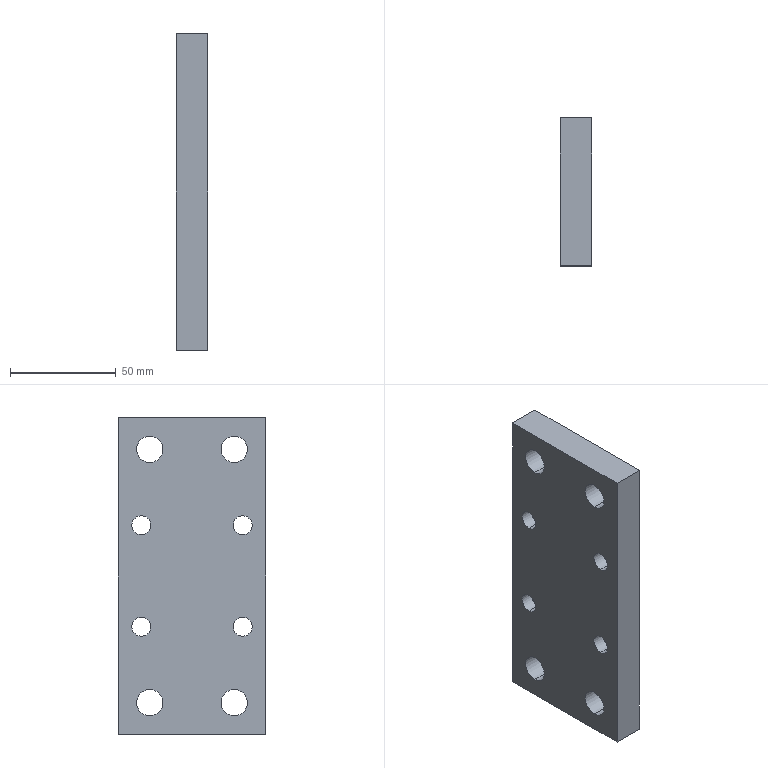Part | SolidWorks | features HoleWzd 2, Extrusion 1 | 1 solid | 34 faces | box 15 x 70 x 150 mm | volume 142248 mm3 | cylinder 24 | plane 10 | commonest cylinder face diameters 9 x8 12.5 x8 15 x8
STEP:
#1=CARTESIAN_POINT('',(15.,20.,-66.25));
#2=VERTEX_POINT('',#1);
#3=CARTESIAN_POINT('',(15.,20.,-53.75));
#4=VERTEX_POINT('',#3);
#5=CARTESIAN_POINT('',(15.,20.,-60.));
#6=DIRECTION('',(-1.,0.,0.));
#7=DIRECTION('',(0.,0.,1.));
#8=AXIS2_PLACEMENT_3D('',#5,#6,#7);
#9=CIRCLE('',#8,6.25);
#10=EDGE_CURVE('',#2,#4,#9,.T.);
#11=ORIENTED_EDGE('',*,*,#10,.F.);
#12=CARTESIAN_POINT('',(0.,20.,-66.25));
#13=VERTEX_POINT('',#12);
#14=CARTESIAN_POINT('',(0.,20.,-66.25));
#15=DIRECTION('',(-1.,0.,0.));
#16=VECTOR('',#15,1000.);
#17=LINE('',#14,#16);
#18=EDGE_CURVE('',#2,#13,#17,.T.);
#19=ORIENTED_EDGE('',*,*,#18,.T.);
#20=CARTESIAN_POINT('',(0.,20.,-53.75));
#21=VERTEX_POINT('',#20);
#22=CARTESIAN_POINT('',(0.,20.,-60.));
#23=DIRECTION('',(-1.,0.,0.));
#24=DIRECTION('',(0.,0.,1.));
#25=AXIS2_PLACEMENT_3D('',#22,#23,#24);
#26=CIRCLE('',#25,6.25);
#27=EDGE_CURVE('',#13,#21,#26,.T.);
#28=ORIENTED_EDGE('',*,*,#27,.T.);
#29=CARTESIAN_POINT('',(0.,20.,-53.75));
#30=DIRECTION('',(-1.,0.,0.));
#31=VECTOR('',#30,1000.);
#32=LINE('',#29,#31);
#33=EDGE_CURVE('',#4,#21,#32,.T.);
#34=ORIENTED_EDGE('',*,*,#33,.F.);
#35=EDGE_LOOP('',(#11,#19,#28,#34));
#36=FACE_OUTER_BOUND('',#35,.T.);
#37=CARTESIAN_POINT('',(0.,20.,-60.));
#38=DIRECTION('',(-1.,0.,0.));
#39=DIRECTION('',(0.,0.,1.));
#40=AXIS2_PLACEMENT_3D('',#37,#38,#39);
#41=CYLINDRICAL_SURFACE('',#40,6.25);
#42=ADVANCED_FACE('',(#36),#41,.F.);
#43=CARTESIAN_POINT('',(15.,-20.,-66.25));
#44=VERTEX_POINT('',#43);
#45=CARTESIAN_POINT('',(15.,-20.,-53.75));
#46=VERTEX_POINT('',#45);
#47=CARTESIAN_POINT('',(15.,-20.,-60.));
#48=DIRECTION('',(-1.,0.,0.));
#49=DIRECTION('',(0.,0.,1.));
#50=AXIS2_PLACEMENT_3D('',#47,#48,#49);
#51=CIRCLE('',#50,6.25);
#52=EDGE_CURVE('',#44,#46,#51,.T.);
#53=ORIENTED_EDGE('',*,*,#52,.F.);
#54=CARTESIAN_POINT('',(0.,-20.,-66.25));
#55=VERTEX_POINT('',#54);
#56=CARTESIAN_POINT('',(0.,-20.,-66.25));
#57=DIRECTION('',(-1.,0.,0.));
#58=VECTOR('',#57,1000.);
#59=LINE('',#56,#58);
#60=EDGE_CURVE('',#44,#55,#59,.T.);
#61=ORIENTED_EDGE('',*,*,#60,.T.);
#62=CARTESIAN_POINT('',(0.,-20.,-53.75));
#63=VERTEX_POINT('',#62);
#64=CARTESIAN_POINT('',(0.,-20.,-60.));
#65=DIRECTION('',(-1.,0.,0.));
#66=DIRECTION('',(0.,0.,1.));
#67=AXIS2_PLACEMENT_3D('',#64,#65,#66);
#68=CIRCLE('',#67,6.25);
#69=EDGE_CURVE('',#55,#63,#68,.T.);
#70=ORIENTED_EDGE('',*,*,#69,.T.);
#71=CARTESIAN_POINT('',(0.,-20.,-53.75));
#72=DIRECTION('',(-1.,0.,0.));
#73=VECTOR('',#72,1000.);
#74=LINE('',#71,#73);
#75=EDGE_CURVE('',#46,#63,#74,.T.);
#76=ORIENTED_EDGE('',*,*,#75,.F.);
#77=EDGE_LOOP('',(#53,#61,#70,#76));
#78=FACE_OUTER_BOUND('',#77,.T.);
#79=CARTESIAN_POINT('',(0.,-20.,-60.));
#80=DIRECTION('',(-1.,0.,0.));
#81=DIRECTION('',(0.,0.,1.));
#82=AXIS2_PLACEMENT_3D('',#79,#80,#81);
#83=CYLINDRICAL_SURFACE('',#82,6.25);
#84=ADVANCED_FACE('',(#78),#83,.F.);
#85=CARTESIAN_POINT('',(15.,20.,53.75));
#86=VERTEX_POINT('',#85);
#87=CARTESIAN_POINT('',(15.,20.,66.25));
#88=VERTEX_POINT('',#87);
#89=CARTESIAN_POINT('',(15.,20.,60.));
#90=DIRECTION('',(-1.,0.,0.));
#91=DIRECTION('',(0.,0.,1.));
#92=AXIS2_PLACEMENT_3D('',#89,#90,#91);
#93=CIRCLE('',#92,6.25);
#94=EDGE_CURVE('',#86,#88,#93,.T.);
#95=ORIENTED_EDGE('',*,*,#94,.F.);
#96=CARTESIAN_POINT('',(0.,20.,53.75));
#97=VERTEX_POINT('',#96);
#98=CARTESIAN_POINT('',(0.,20.,53.75));
#99=DIRECTION('',(-1.,0.,0.));
#100=VECTOR('',#99,1000.);
#101=LINE('',#98,#100);
#102=EDGE_CURVE('',#86,#97,#101,.T.);
#103=ORIENTED_EDGE('',*,*,#102,.T.);
#104=CARTESIAN_POINT('',(0.,20.,66.25));
#105=VERTEX_POINT('',#104);
#106=CARTESIAN_POINT('',(0.,20.,60.));
#107=DIRECTION('',(-1.,0.,0.));
#108=DIRECTION('',(0.,0.,1.));
#109=AXIS2_PLACEMENT_3D('',#106,#107,#108);
#110=CIRCLE('',#109,6.25);
#111=EDGE_CURVE('',#97,#105,#110,.T.);
#112=ORIENTED_EDGE('',*,*,#111,.T.);
#113=CARTESIAN_POINT('',(0.,20.,66.25));
#114=DIRECTION('',(-1.,0.,0.));
#115=VECTOR('',#114,1000.);
#116=LINE('',#113,#115);
#117=EDGE_CURVE('',#88,#105,#116,.T.);
#118=ORIENTED_EDGE('',*,*,#117,.F.);
#119=EDGE_LOOP('',(#95,#103,#112,#118));
#120=FACE_OUTER_BOUND('',#119,.T.);
#121=CARTESIAN_POINT('',(0.,20.,60.));
#122=DIRECTION('',(-1.,0.,0.));
#123=DIRECTION('',(0.,0.,1.));
#124=AXIS2_PLACEMENT_3D('',#121,#122,#123);
#125=CYLINDRICAL_SURFACE('',#124,6.25);
#126=ADVANCED_FACE('',(#120),#125,.F.);
#127=CARTESIAN_POINT('',(15.,-20.,53.75));
#128=VERTEX_POINT('',#127);
#129=CARTESIAN_POINT('',(15.,-20.,66.25));
#130=VERTEX_POINT('',#129);
#131=CARTESIAN_POINT('',(15.,-20.,60.));
#132=DIRECTION('',(-1.,0.,0.));
#133=DIRECTION('',(0.,0.,1.));
#134=AXIS2_PLACEMENT_3D('',#131,#132,#133);
#135=CIRCLE('',#134,6.25);
#136=EDGE_CURVE('',#128,#130,#135,.T.);
#137=ORIENTED_EDGE('',*,*,#136,.F.);
#138=CARTESIAN_POINT('',(0.,-20.,53.75));
#139=VERTEX_POINT('',#138);
#140=CARTESIAN_POINT('',(0.,-20.,53.75));
#141=DIRECTION('',(-1.,0.,0.));
#142=VECTOR('',#141,1000.);
#143=LINE('',#140,#142);
#144=EDGE_CURVE('',#128,#139,#143,.T.);
#145=ORIENTED_EDGE('',*,*,#144,.T.);
#146=CARTESIAN_POINT('',(0.,-20.,66.25));
#147=VERTEX_POINT('',#146);
#148=CARTESIAN_POINT('',(0.,-20.,60.));
#149=DIRECTION('',(-1.,0.,0.));
#150=DIRECTION('',(0.,0.,1.));
#151=AXIS2_PLACEMENT_3D('',#148,#149,#150);
#152=CIRCLE('',#151,6.25);
#153=EDGE_CURVE('',#139,#147,#152,.T.);
#154=ORIENTED_EDGE('',*,*,#153,.T.);
#155=CARTESIAN_POINT('',(0.,-20.,66.25));
#156=DIRECTION('',(-1.,0.,0.));
#157=VECTOR('',#156,1000.);
#158=LINE('',#155,#157);
#159=EDGE_CURVE('',#130,#147,#158,.T.);
#160=ORIENTED_EDGE('',*,*,#159,.F.);
#161=EDGE_LOOP('',(#137,#145,#154,#160));
#162=FACE_OUTER_BOUND('',#161,.T.);
#163=CARTESIAN_POINT('',(0.,-20.,60.));
#164=DIRECTION('',(-1.,0.,0.));
#165=DIRECTION('',(0.,0.,1.));
#166=AXIS2_PLACEMENT_3D('',#163,#164,#165);
#167=CYLINDRICAL_SURFACE('',#166,6.25);
#168=ADVANCED_FACE('',(#162),#167,.F.);
#169=CARTESIAN_POINT('',(6.,24.,31.5));
#170=VERTEX_POINT('',#169);
#171=CARTESIAN_POINT('',(6.,24.,16.5));
#172=VERTEX_POINT('',#171);
#173=CARTESIAN_POINT('',(6.,24.,24.));
#174=DIRECTION('',(1.,0.,0.));
#175=DIRECTION('',(0.,0.,-1.));
#176=AXIS2_PLACEMENT_3D('',#173,#174,#175);
#177=CIRCLE('',#176,7.5);
#178=EDGE_CURVE('',#170,#172,#177,.T.);
#179=ORIENTED_EDGE('',*,*,#178,.F.);
#180=CARTESIAN_POINT('',(15.,24.,31.5));
#181=VERTEX_POINT('',#180);
#182=CARTESIAN_POINT('',(15.,24.,31.5));
#183=DIRECTION('',(1.,0.,0.));
#184=VECTOR('',#183,1000.);
#185=LINE('',#182,#184);
#186=EDGE_CURVE('',#170,#181,#185,.T.);
#187=ORIENTED_EDGE('',*,*,#186,.T.);
#188=CARTESIAN_POINT('',(15.,24.,16.5));
#189=VERTEX_POINT('',#188);
#190=CARTESIAN_POINT('',(15.,24.,24.));
#191=DIRECTION('',(1.,0.,0.));
#192=DIRECTION('',(0.,0.,-1.));
#193=AXIS2_PLACEMENT_3D('',#190,#191,#192);
#194=CIRCLE('',#193,7.5);
#195=EDGE_CURVE('',#181,#189,#194,.T.);
#196=ORIENTED_EDGE('',*,*,#195,.T.);
#197=CARTESIAN_POINT('',(15.,24.,16.5));
#198=DIRECTION('',(1.,0.,0.));
#199=VECTOR('',#198,1000.);
#200=LINE('',#197,#199);
#201=EDGE_CURVE('',#172,#189,#200,.T.);
#202=ORIENTED_EDGE('',*,*,#201,.F.);
#203=EDGE_LOOP('',(#179,#187,#196,#202));
#204=FACE_OUTER_BOUND('',#203,.T.);
#205=CARTESIAN_POINT('',(15.,24.,24.));
#206=DIRECTION('',(1.,0.,0.));
#207=DIRECTION('',(0.,0.,-1.));
#208=AXIS2_PLACEMENT_3D('',#205,#206,#207);
#209=CYLINDRICAL_SURFACE('',#208,7.5);
#210=ADVANCED_FACE('',(#204),#209,.F.);
#211=CARTESIAN_POINT('',(0.,24.,28.5));
#212=VERTEX_POINT('',#211);
#213=CARTESIAN_POINT('',(0.,24.,19.5));
#214=VERTEX_POINT('',#213);
#215=CARTESIAN_POINT('',(0.,24.,24.));
#216=DIRECTION('',(1.,0.,0.));
#217=DIRECTION('',(0.,0.,-1.));
#218=AXIS2_PLACEMENT_3D('',#215,#216,#217);
#219=CIRCLE('',#218,4.5);
#220=EDGE_CURVE('',#212,#214,#219,.T.);
#221=ORIENTED_EDGE('',*,*,#220,.F.);
#222=CARTESIAN_POINT('',(6.,24.,28.5));
#223=VERTEX_POINT('',#222);
#224=CARTESIAN_POINT('',(15.,24.,28.5));
#225=DIRECTION('',(1.,0.,0.));
#226=VECTOR('',#225,1000.);
#227=LINE('',#224,#226);
#228=EDGE_CURVE('',#212,#223,#227,.T.);
#229=ORIENTED_EDGE('',*,*,#228,.T.);
#230=CARTESIAN_POINT('',(6.,24.,19.5));
#231=VERTEX_POINT('',#230);
#232=CARTESIAN_POINT('',(6.,24.,24.));
#233=DIRECTION('',(1.,0.,0.));
#234=DIRECTION('',(0.,0.,-1.));
#235=AXIS2_PLACEMENT_3D('',#232,#233,#234);
#236=CIRCLE('',#235,4.5);
#237=EDGE_CURVE('',#223,#231,#236,.T.);
#238=ORIENTED_EDGE('',*,*,#237,.T.);
#239=CARTESIAN_POINT('',(15.,24.,19.5));
#240=DIRECTION('',(1.,0.,0.));
#241=VECTOR('',#240,1000.);
#242=LINE('',#239,#241);
#243=EDGE_CURVE('',#214,#231,#242,.T.);
#244=ORIENTED_EDGE('',*,*,#243,.F.);
#245=EDGE_LOOP('',(#221,#229,#238,#244));
#246=FACE_OUTER_BOUND('',#245,.T.);
#247=CARTESIAN_POINT('',(15.,24.,24.));
#248=DIRECTION('',(1.,0.,0.));
#249=DIRECTION('',(0.,0.,-1.));
#250=AXIS2_PLACEMENT_3D('',#247,#248,#249);
#251=CYLINDRICAL_SURFACE('',#250,4.5);
#252=ADVANCED_FACE('',(#246),#251,.F.);
#253=CARTESIAN_POINT('',(6.,24.,-16.5));
#254=VERTEX_POINT('',#253);
#255=CARTESIAN_POINT('',(6.,24.,-31.5));
#256=VERTEX_POINT('',#255);
#257=CARTESIAN_POINT('',(6.,24.,-24.));
#258=DIRECTION('',(1.,0.,0.));
#259=DIRECTION('',(0.,0.,-1.));
#260=AXIS2_PLACEMENT_3D('',#257,#258,#259);
#261=CIRCLE('',#260,7.5);
#262=EDGE_CURVE('',#254,#256,#261,.T.);
#263=ORIENTED_EDGE('',*,*,#262,.F.);
#264=CARTESIAN_POINT('',(15.,24.,-16.5));
#265=VERTEX_POINT('',#264);
#266=CARTESIAN_POINT('',(15.,24.,-16.5));
#267=DIRECTION('',(1.,0.,0.));
#268=VECTOR('',#267,1000.);
#269=LINE('',#266,#268);
#270=EDGE_CURVE('',#254,#265,#269,.T.);
#271=ORIENTED_EDGE('',*,*,#270,.T.);
#272=CARTESIAN_POINT('',(15.,24.,-31.5));
#273=VERTEX_POINT('',#272);
#274=CARTESIAN_POINT('',(15.,24.,-24.));
#275=DIRECTION('',(1.,0.,0.));
#276=DIRECTION('',(0.,0.,-1.));
#277=AXIS2_PLACEMENT_3D('',#274,#275,#276);
#278=CIRCLE('',#277,7.5);
#279=EDGE_CURVE('',#265,#273,#278,.T.);
#280=ORIENTED_EDGE('',*,*,#279,.T.);
#281=CARTESIAN_POINT('',(15.,24.,-31.5));
#282=DIRECTION('',(1.,0.,0.));
#283=VECTOR('',#282,1000.);
#284=LINE('',#281,#283);
#285=EDGE_CURVE('',#256,#273,#284,.T.);
#286=ORIENTED_EDGE('',*,*,#285,.F.);
#287=EDGE_LOOP('',(#263,#271,#280,#286));
#288=FACE_OUTER_BOUND('',#287,.T.);
#289=CARTESIAN_POINT('',(15.,24.,-24.));
#290=DIRECTION('',(1.,0.,0.));
#291=DIRECTION('',(0.,0.,-1.));
#292=AXIS2_PLACEMENT_3D('',#289,#290,#291);
#293=CYLINDRICAL_SURFACE('',#292,7.5);
#294=ADVANCED_FACE('',(#288),#293,.F.);
#295=CARTESIAN_POINT('',(0.,24.,-19.5));
#296=VERTEX_POINT('',#295);
#297=CARTESIAN_POINT('',(0.,24.,-28.5));
#298=VERTEX_POINT('',#297);
#299=CARTESIAN_POINT('',(0.,24.,-24.));
#300=DIRECTION('',(1.,0.,0.));
#301=DIRECTION('',(0.,0.,-1.));
#302=AXIS2_PLACEMENT_3D('',#299,#300,#301);
#303=CIRCLE('',#302,4.5);
#304=EDGE_CURVE('',#296,#298,#303,.T.);
#305=ORIENTED_EDGE('',*,*,#304,.F.);
#306=CARTESIAN_POINT('',(6.,24.,-19.5));
#307=VERTEX_POINT('',#306);
#308=CARTESIAN_POINT('',(15.,24.,-19.5));
#309=DIRECTION('',(1.,0.,0.));
#310=VECTOR('',#309,1000.);
#311=LINE('',#308,#310);
#312=EDGE_CURVE('',#296,#307,#311,.T.);
#313=ORIENTED_EDGE('',*,*,#312,.T.);
#314=CARTESIAN_POINT('',(6.,24.,-28.5));
#315=VERTEX_POINT('',#314);
#316=CARTESIAN_POINT('',(6.,24.,-24.));
#317=DIRECTION('',(1.,0.,0.));
#318=DIRECTION('',(0.,0.,-1.));
#319=AXIS2_PLACEMENT_3D('',#316,#317,#318);
#320=CIRCLE('',#319,4.5);
#321=EDGE_CURVE('',#307,#315,#320,.T.);
#322=ORIENTED_EDGE('',*,*,#321,.T.);
#323=CARTESIAN_POINT('',(15.,24.,-28.5));
#324=DIRECTION('',(1.,0.,0.));
#325=VECTOR('',#324,1000.);
#326=LINE('',#323,#325);
#327=EDGE_CURVE('',#298,#315,#326,.T.);
#328=ORIENTED_EDGE('',*,*,#327,.F.);
#329=EDGE_LOOP('',(#305,#313,#322,#328));
#330=FACE_OUTER_BOUND('',#329,.T.);
#331=CARTESIAN_POINT('',(15.,24.,-24.));
#332=DIRECTION('',(1.,0.,0.));
#333=DIRECTION('',(0.,0.,-1.));
#334=AXIS2_PLACEMENT_3D('',#331,#332,#333);
#335=CYLINDRICAL_SURFACE('',#334,4.5);
#336=ADVANCED_FACE('',(#330),#335,.F.);
#337=CARTESIAN_POINT('',(6.,-24.,31.5));
#338=VERTEX_POINT('',#337);
#339=CARTESIAN_POINT('',(6.,-24.,16.5));
#340=VERTEX_POINT('',#339);
#341=CARTESIAN_POINT('',(6.,-24.,24.));
#342=DIRECTION('',(1.,0.,0.));
#343=DIRECTION('',(0.,0.,-1.));
#344=AXIS2_PLACEMENT_3D('',#341,#342,#343);
#345=CIRCLE('',#344,7.5);
#346=EDGE_CURVE('',#338,#340,#345,.T.);
#347=ORIENTED_EDGE('',*,*,#346,.F.);
#348=CARTESIAN_POINT('',(15.,-24.,31.5));
#349=VERTEX_POINT('',#348);
#350=CARTESIAN_POINT('',(15.,-24.,31.5));
#351=DIRECTION('',(1.,0.,0.));
#352=VECTOR('',#351,1000.);
#353=LINE('',#350,#352);
#354=EDGE_CURVE('',#338,#349,#353,.T.);
#355=ORIENTED_EDGE('',*,*,#354,.T.);
#356=CARTESIAN_POINT('',(15.,-24.,16.5));
#357=VERTEX_POINT('',#356);
#358=CARTESIAN_POINT('',(15.,-24.,24.));
#359=DIRECTION('',(1.,0.,0.));
#360=DIRECTION('',(0.,0.,-1.));
#361=AXIS2_PLACEMENT_3D('',#358,#359,#360);
#362=CIRCLE('',#361,7.5);
#363=EDGE_CURVE('',#349,#357,#362,.T.);
#364=ORIENTED_EDGE('',*,*,#363,.T.);
#365=CARTESIAN_POINT('',(15.,-24.,16.5));
#366=DIRECTION('',(1.,0.,0.));
#367=VECTOR('',#366,1000.);
#368=LINE('',#365,#367);
#369=EDGE_CURVE('',#340,#357,#368,.T.);
#370=ORIENTED_EDGE('',*,*,#369,.F.);
#371=EDGE_LOOP('',(#347,#355,#364,#370));
#372=FACE_OUTER_BOUND('',#371,.T.);
#373=CARTESIAN_POINT('',(15.,-24.,24.));
#374=DIRECTION('',(1.,0.,0.));
#375=DIRECTION('',(0.,0.,-1.));
#376=AXIS2_PLACEMENT_3D('',#373,#374,#375);
#377=CYLINDRICAL_SURFACE('',#376,7.5);
#378=ADVANCED_FACE('',(#372),#377,.F.);
#379=CARTESIAN_POINT('',(0.,-24.,28.5));
#380=VERTEX_POINT('',#379);
#381=CARTESIAN_POINT('',(0.,-24.,19.5));
#382=VERTEX_POINT('',#381);
#383=CARTESIAN_POINT('',(0.,-24.,24.));
#384=DIRECTION('',(1.,0.,0.));
#385=DIRECTION('',(0.,0.,-1.));
#386=AXIS2_PLACEMENT_3D('',#383,#384,#385);
#387=CIRCLE('',#386,4.5);
#388=EDGE_CURVE('',#380,#382,#387,.T.);
#389=ORIENTED_EDGE('',*,*,#388,.F.);
#390=CARTESIAN_POINT('',(6.,-24.,28.5));
#391=VERTEX_POINT('',#390);
#392=CARTESIAN_POINT('',(15.,-24.,28.5));
#393=DIRECTION('',(1.,0.,0.));
#394=VECTOR('',#393,1000.);
#395=LINE('',#392,#394);
#396=EDGE_CURVE('',#380,#391,#395,.T.);
#397=ORIENTED_EDGE('',*,*,#396,.T.);
#398=CARTESIAN_POINT('',(6.,-24.,19.5));
#399=VERTEX_POINT('',#398);
#400=CARTESIAN_POINT('',(6.,-24.,24.));
#401=DIRECTION('',(1.,0.,0.));
#402=DIRECTION('',(0.,0.,-1.));
#403=AXIS2_PLACEMENT_3D('',#400,#401,#402);
#404=CIRCLE('',#403,4.5);
#405=EDGE_CURVE('',#391,#399,#404,.T.);
#406=ORIENTED_EDGE('',*,*,#405,.T.);
#407=CARTESIAN_POINT('',(15.,-24.,19.5));
#408=DIRECTION('',(1.,0.,0.));
#409=VECTOR('',#408,1000.);
#410=LINE('',#407,#409);
#411=EDGE_CURVE('',#382,#399,#410,.T.);
#412=ORIENTED_EDGE('',*,*,#411,.F.);
#413=EDGE_LOOP('',(#389,#397,#406,#412));
#414=FACE_OUTER_BOUND('',#413,.T.);
#415=CARTESIAN_POINT('',(15.,-24.,24.));
#416=DIRECTION('',(1.,0.,0.));
#417=DIRECTION('',(0.,0.,-1.));
#418=AXIS2_PLACEMENT_3D('',#415,#416,#417);
#419=CYLINDRICAL_SURFACE('',#418,4.5);
#420=ADVANCED_FACE('',(#414),#419,.F.);
#421=CARTESIAN_POINT('',(6.,-24.,-16.5));
#422=VERTEX_POINT('',#421);
#423=CARTESIAN_POINT('',(6.,-24.,-31.5));
#424=VERTEX_POINT('',#423);
#425=CARTESIAN_POINT('',(6.,-24.,-24.));
#426=DIRECTION('',(1.,0.,0.));
#427=DIRECTION('',(0.,0.,-1.));
#428=AXIS2_PLACEMENT_3D('',#425,#426,#427);
#429=CIRCLE('',#428,7.5);
#430=EDGE_CURVE('',#422,#424,#429,.T.);
#431=ORIENTED_EDGE('',*,*,#430,.F.);
#432=CARTESIAN_POINT('',(15.,-24.,-16.5));
#433=VERTEX_POINT('',#432);
#434=CARTESIAN_POINT('',(15.,-24.,-16.5));
#435=DIRECTION('',(1.,0.,0.));
#436=VECTOR('',#435,1000.);
#437=LINE('',#434,#436);
#438=EDGE_CURVE('',#422,#433,#437,.T.);
#439=ORIENTED_EDGE('',*,*,#438,.T.);
#440=CARTESIAN_POINT('',(15.,-24.,-31.5));
#441=VERTEX_POINT('',#440);
#442=CARTESIAN_POINT('',(15.,-24.,-24.));
#443=DIRECTION('',(1.,0.,0.));
#444=DIRECTION('',(0.,0.,-1.));
#445=AXIS2_PLACEMENT_3D('',#442,#443,#444);
#446=CIRCLE('',#445,7.5);
#447=EDGE_CURVE('',#433,#441,#446,.T.);
#448=ORIENTED_EDGE('',*,*,#447,.T.);
#449=CARTESIAN_POINT('',(15.,-24.,-31.5));
#450=DIRECTION('',(1.,0.,0.));
#451=VECTOR('',#450,1000.);
#452=LINE('',#449,#451);
#453=EDGE_CURVE('',#424,#441,#452,.T.);
#454=ORIENTED_EDGE('',*,*,#453,.F.);
#455=EDGE_LOOP('',(#431,#439,#448,#454));
#456=FACE_OUTER_BOUND('',#455,.T.);
#457=CARTESIAN_POINT('',(15.,-24.,-24.));
#458=DIRECTION('',(1.,0.,0.));
#459=DIRECTION('',(0.,0.,-1.));
#460=AXIS2_PLACEMENT_3D('',#457,#458,#459);
#461=CYLINDRICAL_SURFACE('',#460,7.5);
#462=ADVANCED_FACE('',(#456),#461,.F.);
#463=CARTESIAN_POINT('',(0.,-24.,-19.5));
#464=VERTEX_POINT('',#463);
#465=CARTESIAN_POINT('',(0.,-24.,-28.5));
#466=VERTEX_POINT('',#465);
#467=CARTESIAN_POINT('',(0.,-24.,-24.));
#468=DIRECTION('',(1.,0.,0.));
#469=DIRECTION('',(0.,0.,-1.));
#470=AXIS2_PLACEMENT_3D('',#467,#468,#469);
#471=CIRCLE('',#470,4.5);
#472=EDGE_CURVE('',#464,#466,#471,.T.);
#473=ORIENTED_EDGE('',*,*,#472,.F.);
#474=CARTESIAN_POINT('',(6.,-24.,-19.5));
#475=VERTEX_POINT('',#474);
#476=CARTESIAN_POINT('',(15.,-24.,-19.5));
#477=DIRECTION('',(1.,0.,0.));
#478=VECTOR('',#477,1000.);
#479=LINE('',#476,#478);
#480=EDGE_CURVE('',#464,#475,#479,.T.);
#481=ORIENTED_EDGE('',*,*,#480,.T.);
#482=CARTESIAN_POINT('',(6.,-24.,-28.5));
#483=VERTEX_POINT('',#482);
#484=CARTESIAN_POINT('',(6.,-24.,-24.));
#485=DIRECTION('',(1.,0.,0.));
#486=DIRECTION('',(0.,0.,-1.));
#487=AXIS2_PLACEMENT_3D('',#484,#485,#486);
#488=CIRCLE('',#487,4.5);
#489=EDGE_CURVE('',#475,#483,#488,.T.);
#490=ORIENTED_EDGE('',*,*,#489,.T.);
#491=CARTESIAN_POINT('',(15.,-24.,-28.5));
#492=DIRECTION('',(1.,0.,0.));
#493=VECTOR('',#492,1000.);
#494=LINE('',#491,#493);
#495=EDGE_CURVE('',#466,#483,#494,.T.);
#496=ORIENTED_EDGE('',*,*,#495,.F.);
#497=EDGE_LOOP('',(#473,#481,#490,#496));
#498=FACE_OUTER_BOUND('',#497,.T.);
#499=CARTESIAN_POINT('',(15.,-24.,-24.));
#500=DIRECTION('',(1.,0.,0.));
#501=DIRECTION('',(0.,0.,-1.));
#502=AXIS2_PLACEMENT_3D('',#499,#500,#501);
#503=CYLINDRICAL_SURFACE('',#502,4.5);
#504=ADVANCED_FACE('',(#498),#503,.F.);
#505=CARTESIAN_POINT('',(0.,-35.,-75.));
#506=VERTEX_POINT('',#505);
#507=CARTESIAN_POINT('',(0.,35.,-75.));
#508=VERTEX_POINT('',#507);
#509=CARTESIAN_POINT('',(0.,35.,-75.));
#510=DIRECTION('',(0.,1.,0.));
#511=VECTOR('',#510,1000.);
#512=LINE('',#509,#511);
#513=EDGE_CURVE('',#506,#508,#512,.T.);
#514=ORIENTED_EDGE('',*,*,#513,.T.);
#515=CARTESIAN_POINT('',(15.,35.,-75.));
#516=VERTEX_POINT('',#515);
#517=CARTESIAN_POINT('',(15.,35.,-75.));
#518=DIRECTION('',(-1.,0.,0.));
#519=VECTOR('',#518,1000.);
#520=LINE('',#517,#519);
#521=EDGE_CURVE('',#516,#508,#520,.T.);
#522=ORIENTED_EDGE('',*,*,#521,.F.);
#523=CARTESIAN_POINT('',(15.,-35.,-75.));
#524=VERTEX_POINT('',#523);
#525=CARTESIAN_POINT('',(15.,35.,-75.));
#526=DIRECTION('',(0.,1.,0.));
#527=VECTOR('',#526,1000.);
#528=LINE('',#525,#527);
#529=EDGE_CURVE('',#524,#516,#528,.T.);
#530=ORIENTED_EDGE('',*,*,#529,.F.);
#531=CARTESIAN_POINT('',(15.,-35.,-75.));
#532=DIRECTION('',(-1.,0.,0.));
#533=VECTOR('',#532,1000.);
#534=LINE('',#531,#533);
#535=EDGE_CURVE('',#524,#506,#534,.T.);
#536=ORIENTED_EDGE('',*,*,#535,.T.);
#537=EDGE_LOOP('',(#514,#522,#530,#536));
#538=FACE_OUTER_BOUND('',#537,.T.);
#539=CARTESIAN_POINT('',(15.,35.,-75.));
#540=DIRECTION('',(0.,0.,1.));
#541=DIRECTION('',(0.,-1.,0.));
#542=AXIS2_PLACEMENT_3D('',#539,#540,#541);
#543=PLANE('',#542);
#544=ADVANCED_FACE('',(#538),#543,.F.);
#545=CARTESIAN_POINT('',(0.,35.,75.));
#546=VERTEX_POINT('',#545);
#547=CARTESIAN_POINT('',(0.,35.,75.));
#548=DIRECTION('',(0.,0.,1.));
#549=VECTOR('',#548,1000.);
#550=LINE('',#547,#549);
#551=EDGE_CURVE('',#508,#546,#550,.T.);
#552=ORIENTED_EDGE('',*,*,#551,.T.);
#553=CARTESIAN_POINT('',(15.,35.,75.));
#554=VERTEX_POINT('',#553);
#555=CARTESIAN_POINT('',(15.,35.,75.));
#556=DIRECTION('',(-1.,0.,0.));
#557=VECTOR('',#556,1000.);
#558=LINE('',#555,#557);
#559=EDGE_CURVE('',#554,#546,#558,.T.);
#560=ORIENTED_EDGE('',*,*,#559,.F.);
#561=CARTESIAN_POINT('',(15.,35.,75.));
#562=DIRECTION('',(0.,0.,1.));
#563=VECTOR('',#562,1000.);
#564=LINE('',#561,#563);
#565=EDGE_CURVE('',#516,#554,#564,.T.);
#566=ORIENTED_EDGE('',*,*,#565,.F.);
#567=ORIENTED_EDGE('',*,*,#521,.T.);
#568=EDGE_LOOP('',(#552,#560,#566,#567));
#569=FACE_OUTER_BOUND('',#568,.T.);
#570=CARTESIAN_POINT('',(15.,35.,75.));
#571=DIRECTION('',(0.,-1.,0.));
#572=DIRECTION('',(0.,0.,-1.));
#573=AXIS2_PLACEMENT_3D('',#570,#571,#572);
#574=PLANE('',#573);
#575=ADVANCED_FACE('',(#569),#574,.F.);
#576=CARTESIAN_POINT('',(0.,-35.,75.));
#577=VERTEX_POINT('',#576);
#578=CARTESIAN_POINT('',(0.,35.,75.));
#579=DIRECTION('',(0.,-1.,0.));
#580=VECTOR('',#579,1000.);
#581=LINE('',#578,#580);
#582=EDGE_CURVE('',#546,#577,#581,.T.);
#583=ORIENTED_EDGE('',*,*,#582,.T.);
#584=CARTESIAN_POINT('',(15.,-35.,75.));
#585=VERTEX_POINT('',#584);
#586=CARTESIAN_POINT('',(15.,-35.,75.));
#587=DIRECTION('',(-1.,0.,0.));
#588=VECTOR('',#587,1000.);
#589=LINE('',#586,#588);
#590=EDGE_CURVE('',#585,#577,#589,.T.);
#591=ORIENTED_EDGE('',*,*,#590,.F.);
#592=CARTESIAN_POINT('',(15.,35.,75.));
#593=DIRECTION('',(0.,-1.,0.));
#594=VECTOR('',#593,1000.);
#595=LINE('',#592,#594);
#596=EDGE_CURVE('',#554,#585,#595,.T.);
#597=ORIENTED_EDGE('',*,*,#596,.F.);
#598=ORIENTED_EDGE('',*,*,#559,.T.);
#599=EDGE_LOOP('',(#583,#591,#597,#598));
#600=FACE_OUTER_BOUND('',#599,.T.);
#601=CARTESIAN_POINT('',(15.,35.,75.));
#602=DIRECTION('',(0.,0.,-1.));
#603=DIRECTION('',(0.,1.,0.));
#604=AXIS2_PLACEMENT_3D('',#601,#602,#603);
#605=PLANE('',#604);
#606=ADVANCED_FACE('',(#600),#605,.F.);
#607=CARTESIAN_POINT('',(0.,-35.,75.));
#608=DIRECTION('',(0.,0.,-1.));
#609=VECTOR('',#608,1000.);
#610=LINE('',#607,#609);
#611=EDGE_CURVE('',#577,#506,#610,.T.);
#612=ORIENTED_EDGE('',*,*,#611,.T.);
#613=ORIENTED_EDGE('',*,*,#535,.F.);
#614=CARTESIAN_POINT('',(15.,-35.,75.));
#615=DIRECTION('',(0.,0.,-1.));
#616=VECTOR('',#615,1000.);
#617=LINE('',#614,#616);
#618=EDGE_CURVE('',#585,#524,#617,.T.);
#619=ORIENTED_EDGE('',*,*,#618,.F.);
#620=ORIENTED_EDGE('',*,*,#590,.T.);
#621=EDGE_LOOP('',(#612,#613,#619,#620));
#622=FACE_OUTER_BOUND('',#621,.T.);
#623=CARTESIAN_POINT('',(15.,-35.,75.));
#624=DIRECTION('',(0.,1.,0.));
#625=DIRECTION('',(0.,0.,1.));
#626=AXIS2_PLACEMENT_3D('',#623,#624,#625);
#627=PLANE('',#626);
#628=ADVANCED_FACE('',(#622),#627,.F.);
#629=CARTESIAN_POINT('',(15.,20.,-60.));
#630=DIRECTION('',(-1.,0.,0.));
#631=DIRECTION('',(0.,0.,1.));
#632=AXIS2_PLACEMENT_3D('',#629,#630,#631);
#633=CIRCLE('',#632,6.25);
#634=EDGE_CURVE('',#4,#2,#633,.T.);
#635=ORIENTED_EDGE('',*,*,#634,.T.);
#636=ORIENTED_EDGE('',*,*,#10,.T.);
#637=EDGE_LOOP('',(#635,#636));
#638=FACE_BOUND('',#637,.T.);
#639=CARTESIAN_POINT('',(15.,-20.,-60.));
#640=DIRECTION('',(-1.,0.,0.));
#641=DIRECTION('',(0.,0.,1.));
#642=AXIS2_PLACEMENT_3D('',#639,#640,#641);
#643=CIRCLE('',#642,6.25);
#644=EDGE_CURVE('',#46,#44,#643,.T.);
#645=ORIENTED_EDGE('',*,*,#644,.T.);
#646=ORIENTED_EDGE('',*,*,#52,.T.);
#647=EDGE_LOOP('',(#645,#646));
#648=FACE_BOUND('',#647,.T.);
#649=CARTESIAN_POINT('',(15.,20.,60.));
#650=DIRECTION('',(-1.,0.,0.));
#651=DIRECTION('',(0.,0.,1.));
#652=AXIS2_PLACEMENT_3D('',#649,#650,#651);
#653=CIRCLE('',#652,6.25);
#654=EDGE_CURVE('',#88,#86,#653,.T.);
#655=ORIENTED_EDGE('',*,*,#654,.T.);
#656=ORIENTED_EDGE('',*,*,#94,.T.);
#657=EDGE_LOOP('',(#655,#656));
#658=FACE_BOUND('',#657,.T.);
#659=CARTESIAN_POINT('',(15.,-20.,60.));
#660=DIRECTION('',(-1.,0.,0.));
#661=DIRECTION('',(0.,0.,1.));
#662=AXIS2_PLACEMENT_3D('',#659,#660,#661);
#663=CIRCLE('',#662,6.25);
#664=EDGE_CURVE('',#130,#128,#663,.T.);
#665=ORIENTED_EDGE('',*,*,#664,.T.);
#666=ORIENTED_EDGE('',*,*,#136,.T.);
#667=EDGE_LOOP('',(#665,#666));
#668=FACE_BOUND('',#667,.T.);
#669=CARTESIAN_POINT('',(15.,24.,24.));
#670=DIRECTION('',(1.,0.,0.));
#671=DIRECTION('',(0.,0.,-1.));
#672=AXIS2_PLACEMENT_3D('',#669,#670,#671);
#673=CIRCLE('',#672,7.5);
#674=EDGE_CURVE('',#189,#181,#673,.T.);
#675=ORIENTED_EDGE('',*,*,#674,.F.);
#676=ORIENTED_EDGE('',*,*,#195,.F.);
#677=EDGE_LOOP('',(#675,#676));
#678=FACE_BOUND('',#677,.T.);
#679=CARTESIAN_POINT('',(15.,24.,-24.));
#680=DIRECTION('',(1.,0.,0.));
#681=DIRECTION('',(0.,0.,-1.));
#682=AXIS2_PLACEMENT_3D('',#679,#680,#681);
#683=CIRCLE('',#682,7.5);
#684=EDGE_CURVE('',#273,#265,#683,.T.);
#685=ORIENTED_EDGE('',*,*,#684,.F.);
#686=ORIENTED_EDGE('',*,*,#279,.F.);
#687=EDGE_LOOP('',(#685,#686));
#688=FACE_BOUND('',#687,.T.);
#689=CARTESIAN_POINT('',(15.,-24.,24.));
#690=DIRECTION('',(1.,0.,0.));
#691=DIRECTION('',(0.,0.,-1.));
#692=AXIS2_PLACEMENT_3D('',#689,#690,#691);
#693=CIRCLE('',#692,7.5);
#694=EDGE_CURVE('',#357,#349,#693,.T.);
#695=ORIENTED_EDGE('',*,*,#694,.F.);
#696=ORIENTED_EDGE('',*,*,#363,.F.);
#697=EDGE_LOOP('',(#695,#696));
#698=FACE_BOUND('',#697,.T.);
#699=CARTESIAN_POINT('',(15.,-24.,-24.));
#700=DIRECTION('',(1.,0.,0.));
#701=DIRECTION('',(0.,0.,-1.));
#702=AXIS2_PLACEMENT_3D('',#699,#700,#701);
#703=CIRCLE('',#702,7.5);
#704=EDGE_CURVE('',#441,#433,#703,.T.);
#705=ORIENTED_EDGE('',*,*,#704,.F.);
#706=ORIENTED_EDGE('',*,*,#447,.F.);
#707=EDGE_LOOP('',(#705,#706));
#708=FACE_BOUND('',#707,.T.);
#709=ORIENTED_EDGE('',*,*,#529,.T.);
#710=ORIENTED_EDGE('',*,*,#565,.T.);
#711=ORIENTED_EDGE('',*,*,#596,.T.);
#712=ORIENTED_EDGE('',*,*,#618,.T.);
#713=EDGE_LOOP('',(#709,#710,#711,#712));
#714=FACE_OUTER_BOUND('',#713,.T.);
#715=CARTESIAN_POINT('',(15.,0.,0.));
#716=DIRECTION('',(1.,0.,0.));
#717=DIRECTION('',(0.,0.,-1.));
#718=AXIS2_PLACEMENT_3D('',#715,#716,#717);
#719=PLANE('',#718);
#720=ADVANCED_FACE('',(#638,#648,#658,#668,#678,#688,#698,#708,#714),#719,.T.);
#721=CARTESIAN_POINT('',(0.,20.,-60.));
#722=DIRECTION('',(-1.,0.,0.));
#723=DIRECTION('',(0.,0.,1.));
#724=AXIS2_PLACEMENT_3D('',#721,#722,#723);
#725=CIRCLE('',#724,6.25);
#726=EDGE_CURVE('',#21,#13,#725,.T.);
#727=ORIENTED_EDGE('',*,*,#726,.F.);
#728=ORIENTED_EDGE('',*,*,#27,.F.);
#729=EDGE_LOOP('',(#727,#728));
#730=FACE_BOUND('',#729,.T.);
#731=CARTESIAN_POINT('',(0.,-20.,-60.));
#732=DIRECTION('',(-1.,0.,0.));
#733=DIRECTION('',(0.,0.,1.));
#734=AXIS2_PLACEMENT_3D('',#731,#732,#733);
#735=CIRCLE('',#734,6.25);
#736=EDGE_CURVE('',#63,#55,#735,.T.);
#737=ORIENTED_EDGE('',*,*,#736,.F.);
#738=ORIENTED_EDGE('',*,*,#69,.F.);
#739=EDGE_LOOP('',(#737,#738));
#740=FACE_BOUND('',#739,.T.);
#741=CARTESIAN_POINT('',(0.,20.,60.));
#742=DIRECTION('',(-1.,0.,0.));
#743=DIRECTION('',(0.,0.,1.));
#744=AXIS2_PLACEMENT_3D('',#741,#742,#743);
#745=CIRCLE('',#744,6.25);
#746=EDGE_CURVE('',#105,#97,#745,.T.);
#747=ORIENTED_EDGE('',*,*,#746,.F.);
#748=ORIENTED_EDGE('',*,*,#111,.F.);
#749=EDGE_LOOP('',(#747,#748));
#750=FACE_BOUND('',#749,.T.);
#751=CARTESIAN_POINT('',(0.,-20.,60.));
#752=DIRECTION('',(-1.,0.,0.));
#753=DIRECTION('',(0.,0.,1.));
#754=AXIS2_PLACEMENT_3D('',#751,#752,#753);
#755=CIRCLE('',#754,6.25);
#756=EDGE_CURVE('',#147,#139,#755,.T.);
#757=ORIENTED_EDGE('',*,*,#756,.F.);
#758=ORIENTED_EDGE('',*,*,#153,.F.);
#759=EDGE_LOOP('',(#757,#758));
#760=FACE_BOUND('',#759,.T.);
#761=CARTESIAN_POINT('',(0.,24.,24.));
#762=DIRECTION('',(1.,0.,0.));
#763=DIRECTION('',(0.,0.,-1.));
#764=AXIS2_PLACEMENT_3D('',#761,#762,#763);
#765=CIRCLE('',#764,4.5);
#766=EDGE_CURVE('',#214,#212,#765,.T.);
#767=ORIENTED_EDGE('',*,*,#766,.T.);
#768=ORIENTED_EDGE('',*,*,#220,.T.);
#769=EDGE_LOOP('',(#767,#768));
#770=FACE_BOUND('',#769,.T.);
#771=CARTESIAN_POINT('',(0.,24.,-24.));
#772=DIRECTION('',(1.,0.,0.));
#773=DIRECTION('',(0.,0.,-1.));
#774=AXIS2_PLACEMENT_3D('',#771,#772,#773);
#775=CIRCLE('',#774,4.5);
#776=EDGE_CURVE('',#298,#296,#775,.T.);
#777=ORIENTED_EDGE('',*,*,#776,.T.);
#778=ORIENTED_EDGE('',*,*,#304,.T.);
#779=EDGE_LOOP('',(#777,#778));
#780=FACE_BOUND('',#779,.T.);
#781=CARTESIAN_POINT('',(0.,-24.,24.));
#782=DIRECTION('',(1.,0.,0.));
#783=DIRECTION('',(0.,0.,-1.));
#784=AXIS2_PLACEMENT_3D('',#781,#782,#783);
#785=CIRCLE('',#784,4.5);
#786=EDGE_CURVE('',#382,#380,#785,.T.);
#787=ORIENTED_EDGE('',*,*,#786,.T.);
#788=ORIENTED_EDGE('',*,*,#388,.T.);
#789=EDGE_LOOP('',(#787,#788));
#790=FACE_BOUND('',#789,.T.);
#791=CARTESIAN_POINT('',(0.,-24.,-24.));
#792=DIRECTION('',(1.,0.,0.));
#793=DIRECTION('',(0.,0.,-1.));
#794=AXIS2_PLACEMENT_3D('',#791,#792,#793);
#795=CIRCLE('',#794,4.5);
#796=EDGE_CURVE('',#466,#464,#795,.T.);
#797=ORIENTED_EDGE('',*,*,#796,.T.);
#798=ORIENTED_EDGE('',*,*,#472,.T.);
#799=EDGE_LOOP('',(#797,#798));
#800=FACE_BOUND('',#799,.T.);
#801=ORIENTED_EDGE('',*,*,#513,.F.);
#802=ORIENTED_EDGE('',*,*,#611,.F.);
#803=ORIENTED_EDGE('',*,*,#582,.F.);
#804=ORIENTED_EDGE('',*,*,#551,.F.);
#805=EDGE_LOOP('',(#801,#802,#803,#804));
#806=FACE_OUTER_BOUND('',#805,.T.);
#807=CARTESIAN_POINT('',(0.,0.,0.));
#808=DIRECTION('',(1.,0.,0.));
#809=DIRECTION('',(0.,0.,-1.));
#810=AXIS2_PLACEMENT_3D('',#807,#808,#809);
#811=PLANE('',#810);
#812=ADVANCED_FACE('',(#730,#740,#750,#760,#770,#780,#790,#800,#806),#811,.F.);
#813=ORIENTED_EDGE('',*,*,#480,.F.);
#814=ORIENTED_EDGE('',*,*,#796,.F.);
#815=ORIENTED_EDGE('',*,*,#495,.T.);
#816=CARTESIAN_POINT('',(6.,-24.,-24.));
#817=DIRECTION('',(1.,0.,0.));
#818=DIRECTION('',(0.,0.,-1.));
#819=AXIS2_PLACEMENT_3D('',#816,#817,#818);
#820=CIRCLE('',#819,4.5);
#821=EDGE_CURVE('',#483,#475,#820,.T.);
#822=ORIENTED_EDGE('',*,*,#821,.T.);
#823=EDGE_LOOP('',(#813,#814,#815,#822));
#824=FACE_OUTER_BOUND('',#823,.T.);
#825=CARTESIAN_POINT('',(15.,-24.,-24.));
#826=DIRECTION('',(1.,0.,0.));
#827=DIRECTION('',(0.,0.,-1.));
#828=AXIS2_PLACEMENT_3D('',#825,#826,#827);
#829=CYLINDRICAL_SURFACE('',#828,4.5);
#830=ADVANCED_FACE('',(#824),#829,.F.);
#831=ORIENTED_EDGE('',*,*,#821,.F.);
#832=ORIENTED_EDGE('',*,*,#489,.F.);
#833=EDGE_LOOP('',(#831,#832));
#834=FACE_BOUND('',#833,.T.);
#835=CARTESIAN_POINT('',(6.,-24.,-24.));
#836=DIRECTION('',(1.,0.,0.));
#837=DIRECTION('',(0.,0.,-1.));
#838=AXIS2_PLACEMENT_3D('',#835,#836,#837);
#839=CIRCLE('',#838,7.5);
#840=EDGE_CURVE('',#424,#422,#839,.T.);
#841=ORIENTED_EDGE('',*,*,#840,.T.);
#842=ORIENTED_EDGE('',*,*,#430,.T.);
#843=EDGE_LOOP('',(#841,#842));
#844=FACE_OUTER_BOUND('',#843,.T.);
#845=CARTESIAN_POINT('',(6.,-19.5,-24.));
#846=DIRECTION('',(-1.,0.,0.));
#847=DIRECTION('',(0.,0.,1.));
#848=AXIS2_PLACEMENT_3D('',#845,#846,#847);
#849=PLANE('',#848);
#850=ADVANCED_FACE('',(#834,#844),#849,.F.);
#851=ORIENTED_EDGE('',*,*,#438,.F.);
#852=ORIENTED_EDGE('',*,*,#840,.F.);
#853=ORIENTED_EDGE('',*,*,#453,.T.);
#854=ORIENTED_EDGE('',*,*,#704,.T.);
#855=EDGE_LOOP('',(#851,#852,#853,#854));
#856=FACE_OUTER_BOUND('',#855,.T.);
#857=CARTESIAN_POINT('',(15.,-24.,-24.));
#858=DIRECTION('',(1.,0.,0.));
#859=DIRECTION('',(0.,0.,-1.));
#860=AXIS2_PLACEMENT_3D('',#857,#858,#859);
#861=CYLINDRICAL_SURFACE('',#860,7.5);
#862=ADVANCED_FACE('',(#856),#861,.F.);
#863=ORIENTED_EDGE('',*,*,#396,.F.);
#864=ORIENTED_EDGE('',*,*,#786,.F.);
#865=ORIENTED_EDGE('',*,*,#411,.T.);
#866=CARTESIAN_POINT('',(6.,-24.,24.));
#867=DIRECTION('',(1.,0.,0.));
#868=DIRECTION('',(0.,0.,-1.));
#869=AXIS2_PLACEMENT_3D('',#866,#867,#868);
#870=CIRCLE('',#869,4.5);
#871=EDGE_CURVE('',#399,#391,#870,.T.);
#872=ORIENTED_EDGE('',*,*,#871,.T.);
#873=EDGE_LOOP('',(#863,#864,#865,#872));
#874=FACE_OUTER_BOUND('',#873,.T.);
#875=CARTESIAN_POINT('',(15.,-24.,24.));
#876=DIRECTION('',(1.,0.,0.));
#877=DIRECTION('',(0.,0.,-1.));
#878=AXIS2_PLACEMENT_3D('',#875,#876,#877);
#879=CYLINDRICAL_SURFACE('',#878,4.5);
#880=ADVANCED_FACE('',(#874),#879,.F.);
#881=ORIENTED_EDGE('',*,*,#871,.F.);
#882=ORIENTED_EDGE('',*,*,#405,.F.);
#883=EDGE_LOOP('',(#881,#882));
#884=FACE_BOUND('',#883,.T.);
#885=CARTESIAN_POINT('',(6.,-24.,24.));
#886=DIRECTION('',(1.,0.,0.));
#887=DIRECTION('',(0.,0.,-1.));
#888=AXIS2_PLACEMENT_3D('',#885,#886,#887);
#889=CIRCLE('',#888,7.5);
#890=EDGE_CURVE('',#340,#338,#889,.T.);
#891=ORIENTED_EDGE('',*,*,#890,.T.);
#892=ORIENTED_EDGE('',*,*,#346,.T.);
#893=EDGE_LOOP('',(#891,#892));
#894=FACE_OUTER_BOUND('',#893,.T.);
#895=CARTESIAN_POINT('',(6.,-19.5,24.));
#896=DIRECTION('',(-1.,0.,0.));
#897=DIRECTION('',(0.,0.,1.));
#898=AXIS2_PLACEMENT_3D('',#895,#896,#897);
#899=PLANE('',#898);
#900=ADVANCED_FACE('',(#884,#894),#899,.F.);
#901=ORIENTED_EDGE('',*,*,#354,.F.);
#902=ORIENTED_EDGE('',*,*,#890,.F.);
#903=ORIENTED_EDGE('',*,*,#369,.T.);
#904=ORIENTED_EDGE('',*,*,#694,.T.);
#905=EDGE_LOOP('',(#901,#902,#903,#904));
#906=FACE_OUTER_BOUND('',#905,.T.);
#907=CARTESIAN_POINT('',(15.,-24.,24.));
#908=DIRECTION('',(1.,0.,0.));
#909=DIRECTION('',(0.,0.,-1.));
#910=AXIS2_PLACEMENT_3D('',#907,#908,#909);
#911=CYLINDRICAL_SURFACE('',#910,7.5);
#912=ADVANCED_FACE('',(#906),#911,.F.);
#913=ORIENTED_EDGE('',*,*,#312,.F.);
#914=ORIENTED_EDGE('',*,*,#776,.F.);
#915=ORIENTED_EDGE('',*,*,#327,.T.);
#916=CARTESIAN_POINT('',(6.,24.,-24.));
#917=DIRECTION('',(1.,0.,0.));
#918=DIRECTION('',(0.,0.,-1.));
#919=AXIS2_PLACEMENT_3D('',#916,#917,#918);
#920=CIRCLE('',#919,4.5);
#921=EDGE_CURVE('',#315,#307,#920,.T.);
#922=ORIENTED_EDGE('',*,*,#921,.T.);
#923=EDGE_LOOP('',(#913,#914,#915,#922));
#924=FACE_OUTER_BOUND('',#923,.T.);
#925=CARTESIAN_POINT('',(15.,24.,-24.));
#926=DIRECTION('',(1.,0.,0.));
#927=DIRECTION('',(0.,0.,-1.));
#928=AXIS2_PLACEMENT_3D('',#925,#926,#927);
#929=CYLINDRICAL_SURFACE('',#928,4.5);
#930=ADVANCED_FACE('',(#924),#929,.F.);
#931=ORIENTED_EDGE('',*,*,#921,.F.);
#932=ORIENTED_EDGE('',*,*,#321,.F.);
#933=EDGE_LOOP('',(#931,#932));
#934=FACE_BOUND('',#933,.T.);
#935=CARTESIAN_POINT('',(6.,24.,-24.));
#936=DIRECTION('',(1.,0.,0.));
#937=DIRECTION('',(0.,0.,-1.));
#938=AXIS2_PLACEMENT_3D('',#935,#936,#937);
#939=CIRCLE('',#938,7.5);
#940=EDGE_CURVE('',#256,#254,#939,.T.);
#941=ORIENTED_EDGE('',*,*,#940,.T.);
#942=ORIENTED_EDGE('',*,*,#262,.T.);
#943=EDGE_LOOP('',(#941,#942));
#944=FACE_OUTER_BOUND('',#943,.T.);
#945=CARTESIAN_POINT('',(6.,28.5,-24.));
#946=DIRECTION('',(-1.,0.,0.));
#947=DIRECTION('',(0.,0.,1.));
#948=AXIS2_PLACEMENT_3D('',#945,#946,#947);
#949=PLANE('',#948);
#950=ADVANCED_FACE('',(#934,#944),#949,.F.);
#951=ORIENTED_EDGE('',*,*,#270,.F.);
#952=ORIENTED_EDGE('',*,*,#940,.F.);
#953=ORIENTED_EDGE('',*,*,#285,.T.);
#954=ORIENTED_EDGE('',*,*,#684,.T.);
#955=EDGE_LOOP('',(#951,#952,#953,#954));
#956=FACE_OUTER_BOUND('',#955,.T.);
#957=CARTESIAN_POINT('',(15.,24.,-24.));
#958=DIRECTION('',(1.,0.,0.));
#959=DIRECTION('',(0.,0.,-1.));
#960=AXIS2_PLACEMENT_3D('',#957,#958,#959);
#961=CYLINDRICAL_SURFACE('',#960,7.5);
#962=ADVANCED_FACE('',(#956),#961,.F.);
#963=ORIENTED_EDGE('',*,*,#228,.F.);
#964=ORIENTED_EDGE('',*,*,#766,.F.);
#965=ORIENTED_EDGE('',*,*,#243,.T.);
#966=CARTESIAN_POINT('',(6.,24.,24.));
#967=DIRECTION('',(1.,0.,0.));
#968=DIRECTION('',(0.,0.,-1.));
#969=AXIS2_PLACEMENT_3D('',#966,#967,#968);
#970=CIRCLE('',#969,4.5);
#971=EDGE_CURVE('',#231,#223,#970,.T.);
#972=ORIENTED_EDGE('',*,*,#971,.T.);
#973=EDGE_LOOP('',(#963,#964,#965,#972));
#974=FACE_OUTER_BOUND('',#973,.T.);
#975=CARTESIAN_POINT('',(15.,24.,24.));
#976=DIRECTION('',(1.,0.,0.));
#977=DIRECTION('',(0.,0.,-1.));
#978=AXIS2_PLACEMENT_3D('',#975,#976,#977);
#979=CYLINDRICAL_SURFACE('',#978,4.5);
#980=ADVANCED_FACE('',(#974),#979,.F.);
#981=ORIENTED_EDGE('',*,*,#971,.F.);
#982=ORIENTED_EDGE('',*,*,#237,.F.);
#983=EDGE_LOOP('',(#981,#982));
#984=FACE_BOUND('',#983,.T.);
#985=CARTESIAN_POINT('',(6.,24.,24.));
#986=DIRECTION('',(1.,0.,0.));
#987=DIRECTION('',(0.,0.,-1.));
#988=AXIS2_PLACEMENT_3D('',#985,#986,#987);
#989=CIRCLE('',#988,7.5);
#990=EDGE_CURVE('',#172,#170,#989,.T.);
#991=ORIENTED_EDGE('',*,*,#990,.T.);
#992=ORIENTED_EDGE('',*,*,#178,.T.);
#993=EDGE_LOOP('',(#991,#992));
#994=FACE_OUTER_BOUND('',#993,.T.);
#995=CARTESIAN_POINT('',(6.,28.5,24.));
#996=DIRECTION('',(-1.,0.,0.));
#997=DIRECTION('',(0.,0.,1.));
#998=AXIS2_PLACEMENT_3D('',#995,#996,#997);
#999=PLANE('',#998);
#1000=ADVANCED_FACE('',(#984,#994),#999,.F.);
#1001=ORIENTED_EDGE('',*,*,#186,.F.);
#1002=ORIENTED_EDGE('',*,*,#990,.F.);
#1003=ORIENTED_EDGE('',*,*,#201,.T.);
#1004=ORIENTED_EDGE('',*,*,#674,.T.);
#1005=EDGE_LOOP('',(#1001,#1002,#1003,#1004));
#1006=FACE_OUTER_BOUND('',#1005,.T.);
#1007=CARTESIAN_POINT('',(15.,24.,24.));
#1008=DIRECTION('',(1.,0.,0.));
#1009=DIRECTION('',(0.,0.,-1.));
#1010=AXIS2_PLACEMENT_3D('',#1007,#1008,#1009);
#1011=CYLINDRICAL_SURFACE('',#1010,7.5);
#1012=ADVANCED_FACE('',(#1006),#1011,.F.);
#1013=ORIENTED_EDGE('',*,*,#144,.F.);
#1014=ORIENTED_EDGE('',*,*,#664,.F.);
#1015=ORIENTED_EDGE('',*,*,#159,.T.);
#1016=ORIENTED_EDGE('',*,*,#756,.T.);
#1017=EDGE_LOOP('',(#1013,#1014,#1015,#1016));
#1018=FACE_OUTER_BOUND('',#1017,.T.);
#1019=CARTESIAN_POINT('',(0.,-20.,60.));
#1020=DIRECTION('',(-1.,0.,0.));
#1021=DIRECTION('',(0.,0.,1.));
#1022=AXIS2_PLACEMENT_3D('',#1019,#1020,#1021);
#1023=CYLINDRICAL_SURFACE('',#1022,6.25);
#1024=ADVANCED_FACE('',(#1018),#1023,.F.);
#1025=ORIENTED_EDGE('',*,*,#102,.F.);
#1026=ORIENTED_EDGE('',*,*,#654,.F.);
#1027=ORIENTED_EDGE('',*,*,#117,.T.);
#1028=ORIENTED_EDGE('',*,*,#746,.T.);
#1029=EDGE_LOOP('',(#1025,#1026,#1027,#1028));
#1030=FACE_OUTER_BOUND('',#1029,.T.);
#1031=CARTESIAN_POINT('',(0.,20.,60.));
#1032=DIRECTION('',(-1.,0.,0.));
#1033=DIRECTION('',(0.,0.,1.));
#1034=AXIS2_PLACEMENT_3D('',#1031,#1032,#1033);
#1035=CYLINDRICAL_SURFACE('',#1034,6.25);
#1036=ADVANCED_FACE('',(#1030),#1035,.F.);
#1037=ORIENTED_EDGE('',*,*,#60,.F.);
#1038=ORIENTED_EDGE('',*,*,#644,.F.);
#1039=ORIENTED_EDGE('',*,*,#75,.T.);
#1040=ORIENTED_EDGE('',*,*,#736,.T.);
#1041=EDGE_LOOP('',(#1037,#1038,#1039,#1040));
#1042=FACE_OUTER_BOUND('',#1041,.T.);
#1043=CARTESIAN_POINT('',(0.,-20.,-60.));
#1044=DIRECTION('',(-1.,0.,0.));
#1045=DIRECTION('',(0.,0.,1.));
#1046=AXIS2_PLACEMENT_3D('',#1043,#1044,#1045);
#1047=CYLINDRICAL_SURFACE('',#1046,6.25);
#1048=ADVANCED_FACE('',(#1042),#1047,.F.);
#1049=ORIENTED_EDGE('',*,*,#18,.F.);
#1050=ORIENTED_EDGE('',*,*,#634,.F.);
#1051=ORIENTED_EDGE('',*,*,#33,.T.);
#1052=ORIENTED_EDGE('',*,*,#726,.T.);
#1053=EDGE_LOOP('',(#1049,#1050,#1051,#1052));
#1054=FACE_OUTER_BOUND('',#1053,.T.);
#1055=CARTESIAN_POINT('',(0.,20.,-60.));
#1056=DIRECTION('',(-1.,0.,0.));
#1057=DIRECTION('',(0.,0.,1.));
#1058=AXIS2_PLACEMENT_3D('',#1055,#1056,#1057);
#1059=CYLINDRICAL_SURFACE('',#1058,6.25);
#1060=ADVANCED_FACE('',(#1054),#1059,.F.);
#1061=CLOSED_SHELL('',(#42,#84,#126,#168,#210,#252,#294,#336,#378,#420,#462,#504,#544,#575,#606,#628,#720,#812,#830,#850,#862,#880,#900,#912,#930,#950,#962,#980,#1000,#1012,#1024,#1036,#1048,#1060));
#1062=MANIFOLD_SOLID_BREP('',#1061);
#1063=CARTESIAN_POINT('',(0.,0.,0.));
#1064=DIRECTION('',(0.,0.,1.));
#1065=DIRECTION('',(1.,0.,0.));
#1066=AXIS2_PLACEMENT_3D('',#1063,#1064,#1065);
#1067=(LENGTH_UNIT()NAMED_UNIT(*)SI_UNIT(.MILLI.,.METRE.));
#1068=UNCERTAINTY_MEASURE_WITH_UNIT(LENGTH_MEASURE(0.00001),#1067,'','');
#1069=(NAMED_UNIT(*)PLANE_ANGLE_UNIT()SI_UNIT($,.RADIAN.));
#1070=(NAMED_UNIT(*)SI_UNIT($,.STERADIAN.)SOLID_ANGLE_UNIT());
#1071=(GEOMETRIC_REPRESENTATION_CONTEXT(3)GLOBAL_UNCERTAINTY_ASSIGNED_CONTEXT((#1068))GLOBAL_UNIT_ASSIGNED_CONTEXT((#1067,#1069,#1070))REPRESENTATION_CONTEXT('',''));
#1072=ADVANCED_BREP_SHAPE_REPRESENTATION('',(#1062,#1066),#1071);